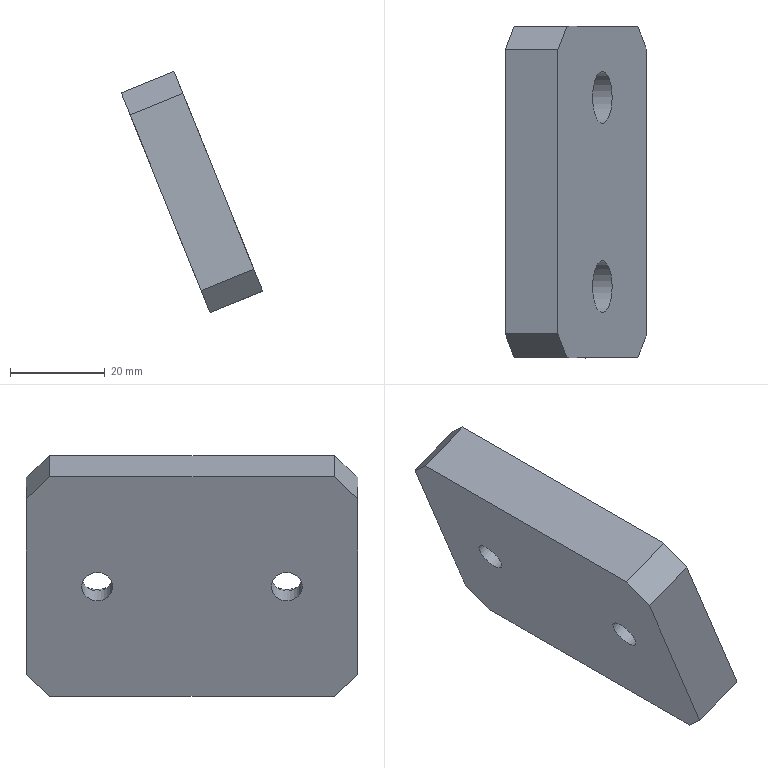Part | STEP file | lll_id442_x_t | 1 solid | 116 faces | box 29.857 x 70 x 50.854 mm | volume 39790 mm3 | plane 58 | other 54 | cylinder 4 | commonest cylinder face diameters 6.5 x2 11 x2